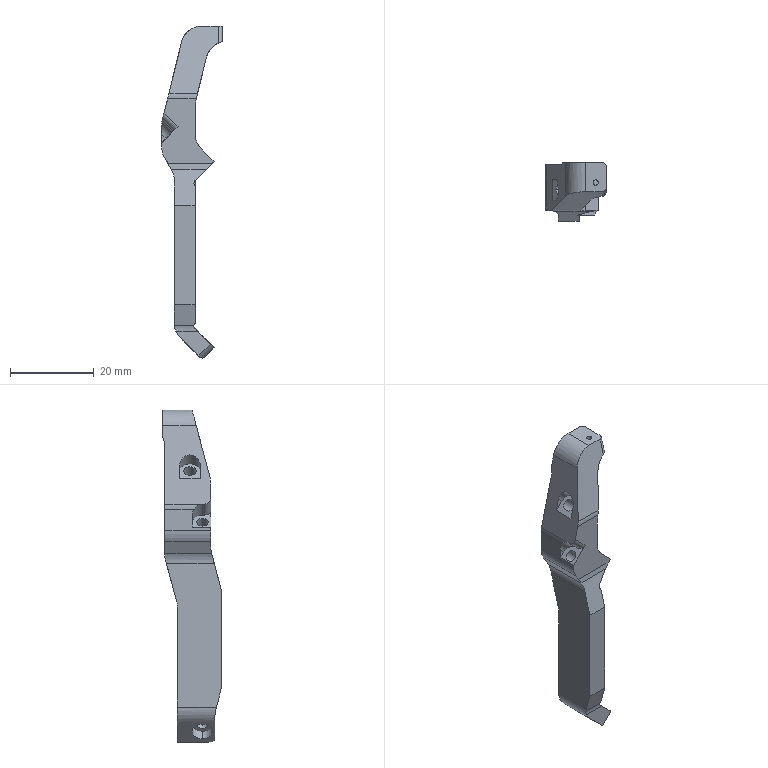CAM job | NX | 3+2 milling, 5-axis milling, drilling | part box 14.5 x 14 x 79.438 mm | stock box 16.1 x 19.5 x 87.438 mm
Tools:
number,name,description,diameter,corner_radius,flute_length,length,flutes
11,D2-7-D2-50-3T,D2-7-D2-50-3T,2.0,0.0,7.0,50.0,2
4,D4-12-D4-50-3T-ROUGH,D4-12-D4-50-3T-粗,4.0,0.0,12.0,50.0,2
5,D4-12-D4-50-3T-FINISH,D4-12-D4-50-3T,4.0,0.0,12.0,50.0,3
2,D6-18-D6-50-3T-ROUGH,D6-18-D6-50-3T-粗,6.0,0.0,18.0,50.0,2
3,D6-18-D6-50-3T-FINISH,D6-18-D6-50-3T,6.0,0.0,18.0,50.0,3
1,D8-25-D8-60-3T-ROUGH,D8-25-D8-60-3T-粗,8.0,0.0,25.0,60.0,2
8,钻头D2.7-39-67,钻刀D2.75-39-67,2.7,0.0,39.0,67.0,2
7,钻头D3.0-42-71,钻刀D3.0-42-71,3.0,0.0,42.0,71.0,2
6,倒角D4-90度,倒角D4-90度,4.0,0.0,5.0,50.0,2
9,球刀R1.25-4-D4-50,球刀R1-4-D4-50,2.5,1.25,4.0,4.5,2
12,D1.3钻头,Drilling Tool,1.3,0.0,35.0,80.0,2
13,M1.6螺纹铣刀,Thread Mill,1.15,0.0,6.5,50.0,1
0,MILL,Milling Tool-5 Parameters,3.0,0.5,50.0,75.0,2
Operations:
program,operation,operation_type,tool,method,geometry_group,spindle_rpm,surface_speed,feed_per_tooth,feed_cut,feed_plunge,cut_length_mm,path_length_mm,cut_time_min,machine_time_min
A1,动态粗,CavityMilling,D8-25-D8-60-3T-ROUGH,METHOD,WORKPIECE_54,4500.0,113.0,0.2222,2000.0,100.0,15697.312,19907.179,5.383,5.804
A1,动态粗_COPY,CavityMilling,D6-18-D6-50-3T-ROUGH,METHOD,WORKPIECE_54,4500.0,84.0,0.1667,1500.0,100.0,1415.828,2943.815,0.941,1.094
A1,PLANAR_MILL_1,PlanarMilling,D4-12-D4-50-3T-ROUGH,METHOD,WORKPIECE_54,3000.0,37.0,0.0667,400.0,100.0,648.996,747.419,1.623,1.632
A1,PLANAR_MILL_1_COPY,PlanarMilling,D4-12-D4-50-3T-ROUGH,METHOD,WORKPIECE_54,3000.0,37.0,0.0667,400.0,100.0,978.788,1619.128,2.447,2.511
A1,PLANAR_MILL_1_COPY_1,PlanarMilling,D4-12-D4-50-3T-FINISH,METHOD,WORKPIECE_54,3000.0,37.0,0.0667,600.0,100.0,37.4,180.376,0.0623,0.0766
A1,PLANAR_MILL_1_COPY_COPY,PlanarMilling,D4-12-D4-50-3T-FINISH,METHOD,WORKPIECE_54,3000.0,37.0,0.0667,600.0,100.0,39.151,220.56,0.0653,0.0834
A1,FLOOR_FACING_COPY,VolumeBased25DMillingOperation,D4-12-D4-50-3T-FINISH,METHOD,A-G54,3000.0,37.0,0.0667,600.0,100.0,421.215,558.015,0.702,0.7157
A1,FLOOR_FACING_COPY_COPY,VolumeBased25DMillingOperation,D4-12-D4-50-3T-FINISH,METHOD,A-G54,3000.0,37.0,0.0667,600.0,100.0,210.707,277.807,0.3512,0.3579
A1,PLANAR_MILL_3,PlanarMilling,D4-12-D4-50-3T-FINISH,METHOD,A-G54,3000.0,37.0,0.0667,600.0,100.0,44.11,98.21,0.0735,0.0789
A1,SPOT_DRILLING_1,HoleDrilling,倒角D4-90度,METHOD,WORKPIECE_54,2500.0,31.0,0.016,80.0,100.0,7.6,69.6,0.095,0.1012
A1,SPOT_DRILLING,HoleDrilling,倒角D4-90度,METHOD,WORKPIECE_54,2500.0,31.0,0.016,80.0,100.0,10.0,94.442,0.125,0.1334
A1,SPOT_DRILLING_COPY,HoleDrilling,倒角D4-90度,METHOD,WORKPIECE_54,2500.0,31.0,0.016,80.0,100.0,8.0,108.442,0.1,0.11
A1,SPOT_DRILLING_2,HoleDrilling,倒角D4-90度,METHOD,WORKPIECE_54,2500.0,31.0,0.016,80.0,100.0,8.0,81.928,0.1,0.1074
A1,SPOT_DRILLING_COPY_1,HoleDrilling,钻头D3.0-42-71,METHOD,WORKPIECE_54,2000.0,18.0,0.01,40.0,100.0,330.0,414.442,8.25,8.258
A1,SPOT_DRILLING_COPY_COPY,HoleDrilling,钻头D2.7-39-67,METHOD,WORKPIECE_54,2000.0,18.0,0.01,40.0,100.0,294.0,394.442,7.35,7.36
A1,SPOT_DRILLING_2_COPY,HoleDrilling,钻头D2.7-39-67,METHOD,WORKPIECE_54,2000.0,18.0,0.01,40.0,100.0,78.0,151.928,1.95,1.957
A1,PLANAR_MILL_2,PlanarMilling,D4-12-D4-50-3T-ROUGH,METHOD,A-G54,3000.0,37.0,0.05,300.0,100.0,133.964,194.364,0.4465,0.4526
A1,PLANAR_MILL,PlanarMilling,D6-18-D6-50-3T-FINISH,METHOD,A-G54,3000.0,56.0,0.0667,600.0,100.0,197.677,461.889,0.3295,0.3559
A1,PLANAR_MILL_COPY,PlanarMilling,D6-18-D6-50-3T-FINISH,METHOD,A-G54,3000.0,56.0,0.0667,600.0,100.0,416.977,502.977,0.695,0.7036
A1,PLANAR_MILL_COPY_COPY,PlanarMilling,D6-18-D6-50-3T-FINISH,METHOD,A-G54,3000.0,56.0,0.0667,600.0,100.0,73.912,257.772,0.1232,0.1416
A1,PLANAR_MILL_4,PlanarMilling,D6-18-D6-50-3T-FINISH,METHOD,A-G54,3000.0,56.0,0.0667,600.0,100.0,47.723,173.654,0.0795,0.0921
A1,3_AXIS_DEBURRING,TpMultiAxisDeburring,球刀R1.25-4-D4-50,METHOD,A-G54,4500.0,28.0,0.1111,1000.0,90.0,205.675,258.612,0.2062,0.2062
A1,CURVE_DRIVE,SurfaceContour,球刀R1.25-4-D4-50,METHOD,A-G54,4500.0,28.0,0.1667,1500.0,90.0,177.581,245.671,0.1187,0.1255
A1,CURVE_DRIVE_COPY,SurfaceContour,球刀R1.25-4-D4-50,METHOD,A-G54,4500.0,28.0,0.1667,1500.0,90.0,164.565,222.824,0.11,0.1158
A1,ZLEVEL_PROFILE_STEEP,ZLevelMilling,MILL,METHOD,A-G54,3500.0,32.0,0.2857,2000.0,100.0,1248.617,1312.576,0.6243,0.6307
A1,DRILLING,Operation,D2-7-D2-50-3T,METHOD,A-G54,3000.0,18.0,0.0033,20.0,0.0,9.274,21.548,0.4637,0.4649
A1,SPOT_DRILLING_3,HoleDrilling,D1.3钻头,METHOD,A-G54,1600.0,6.0,0.0031,10.0,100.0,189.0,243.0,18.9,18.905
A1,THREAD_MILLING,ThreadMilling,M1.6螺纹铣刀,METHOD,A-G54,3500.0,12.0,0.0029,10.0,100.0,182.571,297.568,18.257,18.269
A1,PLANAR_MILL_5,PlanarMilling,D8-25-D8-60-3T-ROUGH,METHOD,A-G54,3000.0,75.0,0.4167,2500.0,100.0,4381.426,11092.72,1.753,2.424
A1,PLANAR_MILL_5_COPY,PlanarMilling,D8-25-D8-60-3T-ROUGH,METHOD,A-G54,3000.0,75.0,0.4167,2500.0,100.0,3770.065,9487.145,1.508,2.08
A1,PLANAR_MILL_5_COPY_COPY,PlanarMilling,D4-12-D4-50-3T-ROUGH,METHOD,A-G54,3000.0,75.0,0.25,1500.0,100.0,281.681,619.897,0.1878,0.2216
B1,PLANAR_MILL_6,PlanarMilling,D8-25-D8-60-3T-ROUGH,METHOD,B-G55,3000.0,56.0,0.2222,2000.0,100.0,7641.629,17408.795,3.821,4.798
B1,PLANAR_MILL_6_COPY,PlanarMilling,D6-18-D6-50-3T-FINISH,METHOD,B-G55,3000.0,56.0,0.0667,600.0,100.0,195.783,388.888,0.3263,0.3456
C1,CURVE_DRIVE_COPY_1,SurfaceContour,球刀R1.25-4-D4-50,METHOD,GZ1,4500.0,28.0,0.1667,1500.0,90.0,170.398,195.412,0.1139,0.1164
C1,3_AXIS_DEBURRING_COPY,TpMultiAxisDeburring,球刀R1.25-4-D4-50,METHOD,GZ1,4500.0,28.0,0.1111,1000.0,90.0,183.126,208.803,0.1833,0.1833
工装1,PLANAR_MILL_7,PlanarMilling,D6-18-D6-50-3T-FINISH,METHOD,GZ1,4500.0,84.0,0.0741,1000.0,100.0,1129.049,2484.176,1.129,1.265
工装1,PLANAR_MILL_7_COPY,PlanarMilling,D6-18-D6-50-3T-FINISH,METHOD,GZ1,4500.0,84.0,0.0444,600.0,100.0,95.188,141.188,0.1586,0.1632